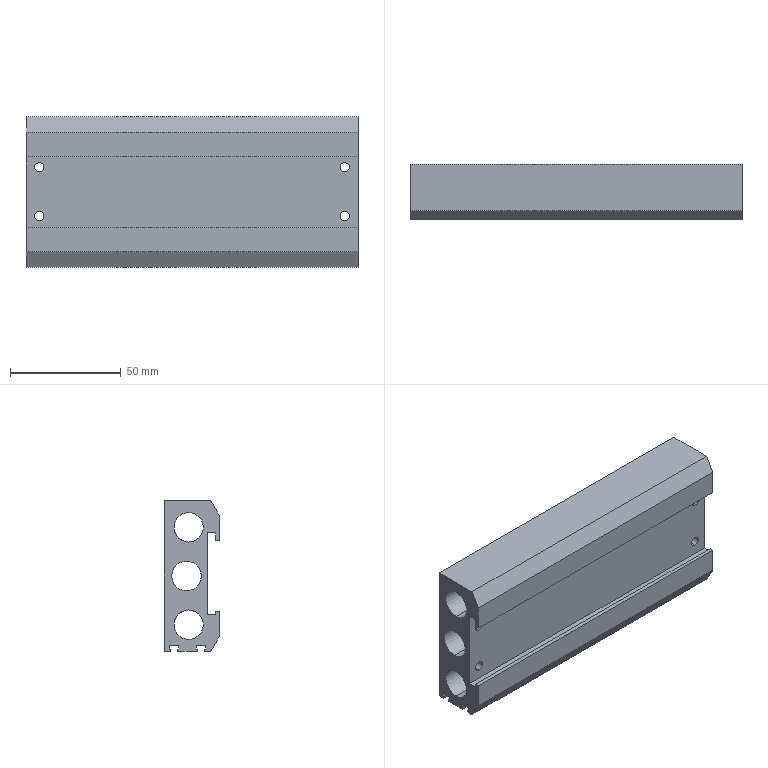Part | STEP file | 8mmM4RD2-8 | 1 solid | 174 faces | box 150 x 25 x 68 mm | volume 146651 mm3 | cylinder 110 | plane 64 | commonest cylinder face diameters 2.85 x32 4 x32 7.5 x32 4.2 x8 13.29 x6